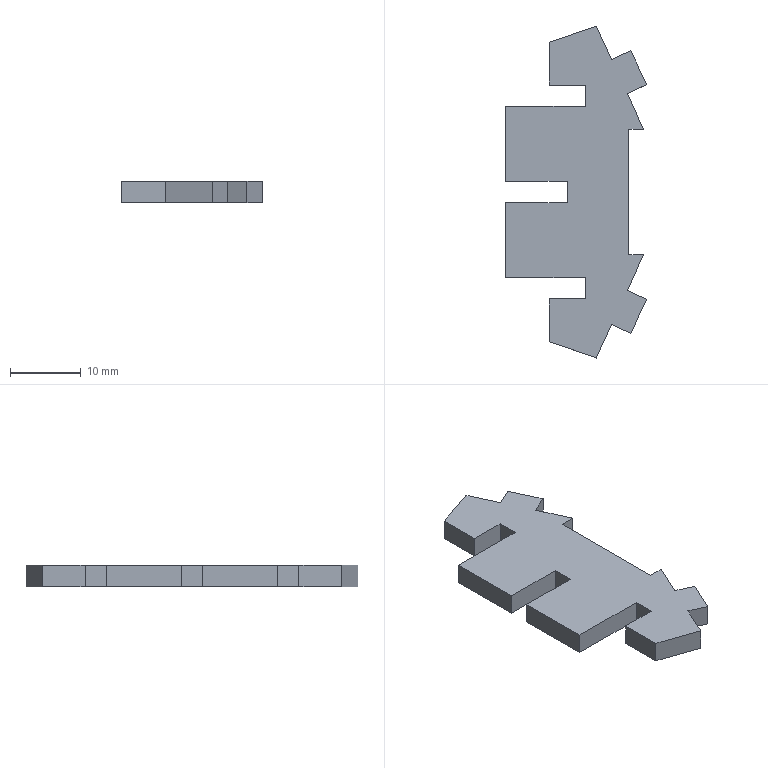Part | SolidWorks | features BaseBody 1 | 1 solid | 30 faces | box 19.907 x 46.828 x 3 mm | volume 1794 mm3 | plane 30
STEP:
#1=CARTESIAN_POINT('',(19.6,-8.833,-1.5));
#2=VERTEX_POINT('',#1);
#3=CARTESIAN_POINT('',(17.493,-8.833,-1.5));
#4=VERTEX_POINT('',#3);
#5=CARTESIAN_POINT('',(0.,-8.833,-1.5));
#6=DIRECTION('',(-1.,0.,0.));
#7=VECTOR('',#6,1000.);
#8=LINE('',#5,#7);
#9=EDGE_CURVE('',#2,#4,#8,.T.);
#10=ORIENTED_EDGE('',*,*,#9,.F.);
#11=CARTESIAN_POINT('',(17.284,-13.888,-1.5));
#12=VERTEX_POINT('',#11);
#13=CARTESIAN_POINT('',(19.544,-8.956,-1.5));
#14=DIRECTION('',(0.4166,0.9091,0.));
#15=VECTOR('',#14,1000.);
#16=LINE('',#13,#15);
#17=EDGE_CURVE('',#12,#2,#16,.T.);
#18=ORIENTED_EDGE('',*,*,#17,.F.);
#19=CARTESIAN_POINT('',(20.008,-15.138,-1.5));
#20=VERTEX_POINT('',#19);
#21=CARTESIAN_POINT('',(-2.257,-4.916,-1.5));
#22=DIRECTION('',(-0.9088,0.4172,0.));
#23=VECTOR('',#22,1000.);
#24=LINE('',#21,#23);
#25=EDGE_CURVE('',#20,#12,#24,.T.);
#26=ORIENTED_EDGE('',*,*,#25,.F.);
#27=CARTESIAN_POINT('',(17.807,-19.931,-1.5));
#28=VERTEX_POINT('',#27);
#29=CARTESIAN_POINT('',(22.265,-10.222,-1.5));
#30=DIRECTION('',(0.4172,0.9088,0.));
#31=VECTOR('',#30,1000.);
#32=LINE('',#29,#31);
#33=EDGE_CURVE('',#28,#20,#32,.T.);
#34=ORIENTED_EDGE('',*,*,#33,.F.);
#35=CARTESIAN_POINT('',(15.086,-18.681,-1.5));
#36=VERTEX_POINT('',#35);
#37=CARTESIAN_POINT('',(-4.457,-9.708,-1.5));
#38=DIRECTION('',(0.9088,-0.4172,0.));
#39=VECTOR('',#38,1000.);
#40=LINE('',#37,#39);
#41=EDGE_CURVE('',#36,#28,#40,.T.);
#42=ORIENTED_EDGE('',*,*,#41,.F.);
#43=CARTESIAN_POINT('',(12.915,-23.414,-1.5));
#44=VERTEX_POINT('',#43);
#45=CARTESIAN_POINT('',(19.544,-8.968,-1.5));
#46=DIRECTION('',(0.4171,0.9089,0.));
#47=VECTOR('',#46,1000.);
#48=LINE('',#45,#47);
#49=EDGE_CURVE('',#44,#36,#48,.T.);
#50=ORIENTED_EDGE('',*,*,#49,.F.);
#51=CARTESIAN_POINT('',(6.282,-21.117,-1.5));
#52=VERTEX_POINT('',#51);
#53=CARTESIAN_POINT('',(-5.857,-16.914,-1.5));
#54=DIRECTION('',(0.9449,-0.3272,0.));
#55=VECTOR('',#54,1000.);
#56=LINE('',#53,#55);
#57=EDGE_CURVE('',#52,#44,#56,.T.);
#58=ORIENTED_EDGE('',*,*,#57,.F.);
#59=CARTESIAN_POINT('',(6.282,-15.081,-1.5));
#60=VERTEX_POINT('',#59);
#61=CARTESIAN_POINT('',(6.282,0.,-1.5));
#62=DIRECTION('',(0.,-1.,0.));
#63=VECTOR('',#62,1000.);
#64=LINE('',#61,#63);
#65=EDGE_CURVE('',#60,#52,#64,.T.);
#66=ORIENTED_EDGE('',*,*,#65,.F.);
#67=CARTESIAN_POINT('',(11.376,-15.081,-1.5));
#68=VERTEX_POINT('',#67);
#69=CARTESIAN_POINT('',(0.,-15.081,-1.5));
#70=DIRECTION('',(-1.,0.,0.));
#71=VECTOR('',#70,1000.);
#72=LINE('',#69,#71);
#73=EDGE_CURVE('',#68,#60,#72,.T.);
#74=ORIENTED_EDGE('',*,*,#73,.F.);
#75=CARTESIAN_POINT('',(11.376,-12.086,-1.5));
#76=VERTEX_POINT('',#75);
#77=CARTESIAN_POINT('',(11.376,0.,-1.5));
#78=DIRECTION('',(0.,-1.,0.));
#79=VECTOR('',#78,1000.);
#80=LINE('',#77,#79);
#81=EDGE_CURVE('',#76,#68,#80,.T.);
#82=ORIENTED_EDGE('',*,*,#81,.F.);
#83=CARTESIAN_POINT('',(0.1003,-12.086,-1.5));
#84=VERTEX_POINT('',#83);
#85=CARTESIAN_POINT('',(0.,-12.086,-1.5));
#86=DIRECTION('',(1.,0.,0.));
#87=VECTOR('',#86,1000.);
#88=LINE('',#85,#87);
#89=EDGE_CURVE('',#84,#76,#88,.T.);
#90=ORIENTED_EDGE('',*,*,#89,.F.);
#91=CARTESIAN_POINT('',(0.1003,-1.498,-1.5));
#92=VERTEX_POINT('',#91);
#93=CARTESIAN_POINT('',(0.1003,0.,-1.5));
#94=DIRECTION('',(0.,1.,0.));
#95=VECTOR('',#94,1000.);
#96=LINE('',#93,#95);
#97=EDGE_CURVE('',#84,#92,#96,.T.);
#98=ORIENTED_EDGE('',*,*,#97,.T.);
#99=CARTESIAN_POINT('',(8.819,-1.498,-1.5));
#100=VERTEX_POINT('',#99);
#101=CARTESIAN_POINT('',(0.,-1.498,-1.5));
#102=DIRECTION('',(-1.,0.,0.));
#103=VECTOR('',#102,1000.);
#104=LINE('',#101,#103);
#105=EDGE_CURVE('',#100,#92,#104,.T.);
#106=ORIENTED_EDGE('',*,*,#105,.F.);
#107=CARTESIAN_POINT('',(8.819,1.498,-1.5));
#108=VERTEX_POINT('',#107);
#109=CARTESIAN_POINT('',(8.819,0.,-1.5));
#110=DIRECTION('',(0.,-1.,0.));
#111=VECTOR('',#110,1000.);
#112=LINE('',#109,#111);
#113=EDGE_CURVE('',#108,#100,#112,.T.);
#114=ORIENTED_EDGE('',*,*,#113,.F.);
#115=CARTESIAN_POINT('',(0.1003,1.498,-1.5));
#116=VERTEX_POINT('',#115);
#117=CARTESIAN_POINT('',(0.,1.498,-1.5));
#118=DIRECTION('',(1.,0.,0.));
#119=VECTOR('',#118,1000.);
#120=LINE('',#117,#119);
#121=EDGE_CURVE('',#116,#108,#120,.T.);
#122=ORIENTED_EDGE('',*,*,#121,.F.);
#123=CARTESIAN_POINT('',(0.1003,12.086,-1.5));
#124=VERTEX_POINT('',#123);
#125=CARTESIAN_POINT('',(0.1003,0.,-1.5));
#126=DIRECTION('',(0.,1.,0.));
#127=VECTOR('',#126,1000.);
#128=LINE('',#125,#127);
#129=EDGE_CURVE('',#116,#124,#128,.T.);
#130=ORIENTED_EDGE('',*,*,#129,.T.);
#131=CARTESIAN_POINT('',(11.376,12.086,-1.5));
#132=VERTEX_POINT('',#131);
#133=CARTESIAN_POINT('',(0.,12.086,-1.5));
#134=DIRECTION('',(-1.,0.,0.));
#135=VECTOR('',#134,1000.);
#136=LINE('',#133,#135);
#137=EDGE_CURVE('',#132,#124,#136,.T.);
#138=ORIENTED_EDGE('',*,*,#137,.F.);
#139=CARTESIAN_POINT('',(11.376,15.081,-1.5));
#140=VERTEX_POINT('',#139);
#141=CARTESIAN_POINT('',(11.376,0.,-1.5));
#142=DIRECTION('',(0.,-1.,0.));
#143=VECTOR('',#142,1000.);
#144=LINE('',#141,#143);
#145=EDGE_CURVE('',#140,#132,#144,.T.);
#146=ORIENTED_EDGE('',*,*,#145,.F.);
#147=CARTESIAN_POINT('',(6.282,15.081,-1.5));
#148=VERTEX_POINT('',#147);
#149=CARTESIAN_POINT('',(0.,15.081,-1.5));
#150=DIRECTION('',(1.,0.,0.));
#151=VECTOR('',#150,1000.);
#152=LINE('',#149,#151);
#153=EDGE_CURVE('',#148,#140,#152,.T.);
#154=ORIENTED_EDGE('',*,*,#153,.F.);
#155=CARTESIAN_POINT('',(6.282,21.117,-1.5));
#156=VERTEX_POINT('',#155);
#157=CARTESIAN_POINT('',(6.282,0.,-1.5));
#158=DIRECTION('',(0.,-1.,0.));
#159=VECTOR('',#158,1000.);
#160=LINE('',#157,#159);
#161=EDGE_CURVE('',#156,#148,#160,.T.);
#162=ORIENTED_EDGE('',*,*,#161,.F.);
#163=CARTESIAN_POINT('',(12.915,23.414,-1.5));
#164=VERTEX_POINT('',#163);
#165=CARTESIAN_POINT('',(-5.857,16.914,-1.5));
#166=DIRECTION('',(-0.9449,-0.3272,0.));
#167=VECTOR('',#166,1000.);
#168=LINE('',#165,#167);
#169=EDGE_CURVE('',#164,#156,#168,.T.);
#170=ORIENTED_EDGE('',*,*,#169,.F.);
#171=CARTESIAN_POINT('',(15.086,18.681,-1.5));
#172=VERTEX_POINT('',#171);
#173=CARTESIAN_POINT('',(19.544,8.968,-1.5));
#174=DIRECTION('',(-0.4171,0.9089,0.));
#175=VECTOR('',#174,1000.);
#176=LINE('',#173,#175);
#177=EDGE_CURVE('',#172,#164,#176,.T.);
#178=ORIENTED_EDGE('',*,*,#177,.F.);
#179=CARTESIAN_POINT('',(17.807,19.931,-1.5));
#180=VERTEX_POINT('',#179);
#181=CARTESIAN_POINT('',(-4.457,9.708,-1.5));
#182=DIRECTION('',(-0.9088,-0.4172,0.));
#183=VECTOR('',#182,1000.);
#184=LINE('',#181,#183);
#185=EDGE_CURVE('',#180,#172,#184,.T.);
#186=ORIENTED_EDGE('',*,*,#185,.F.);
#187=CARTESIAN_POINT('',(20.008,15.138,-1.5));
#188=VERTEX_POINT('',#187);
#189=CARTESIAN_POINT('',(22.265,10.222,-1.5));
#190=DIRECTION('',(-0.4172,0.9088,0.));
#191=VECTOR('',#190,1000.);
#192=LINE('',#189,#191);
#193=EDGE_CURVE('',#188,#180,#192,.T.);
#194=ORIENTED_EDGE('',*,*,#193,.F.);
#195=CARTESIAN_POINT('',(17.284,13.888,-1.5));
#196=VERTEX_POINT('',#195);
#197=CARTESIAN_POINT('',(-2.257,4.916,-1.5));
#198=DIRECTION('',(0.9088,0.4172,0.));
#199=VECTOR('',#198,1000.);
#200=LINE('',#197,#199);
#201=EDGE_CURVE('',#196,#188,#200,.T.);
#202=ORIENTED_EDGE('',*,*,#201,.F.);
#203=CARTESIAN_POINT('',(19.6,8.833,-1.5));
#204=VERTEX_POINT('',#203);
#205=CARTESIAN_POINT('',(19.544,8.956,-1.5));
#206=DIRECTION('',(-0.4166,0.9091,0.));
#207=VECTOR('',#206,1000.);
#208=LINE('',#205,#207);
#209=EDGE_CURVE('',#204,#196,#208,.T.);
#210=ORIENTED_EDGE('',*,*,#209,.F.);
#211=CARTESIAN_POINT('',(17.493,8.833,-1.5));
#212=VERTEX_POINT('',#211);
#213=CARTESIAN_POINT('',(0.,8.833,-1.5));
#214=DIRECTION('',(1.,0.,0.));
#215=VECTOR('',#214,1000.);
#216=LINE('',#213,#215);
#217=EDGE_CURVE('',#212,#204,#216,.T.);
#218=ORIENTED_EDGE('',*,*,#217,.F.);
#219=CARTESIAN_POINT('',(17.493,0.,-1.5));
#220=DIRECTION('',(0.,1.,0.));
#221=VECTOR('',#220,1000.);
#222=LINE('',#219,#221);
#223=EDGE_CURVE('',#4,#212,#222,.T.);
#224=ORIENTED_EDGE('',*,*,#223,.F.);
#225=EDGE_LOOP('',(#10,#18,#26,#34,#42,#50,#58,#66,#74,#82,#90,#98,#106,#114,#122,#130,#138,#146,#154,#162,#170,#178,#186,#194,#202,#210,#218,#224));
#226=FACE_OUTER_BOUND('',#225,.T.);
#227=CARTESIAN_POINT('',(0.,0.,-1.5));
#228=DIRECTION('',(0.,0.,1.));
#229=DIRECTION('',(1.,0.,0.));
#230=AXIS2_PLACEMENT_3D('',#227,#228,#229);
#231=PLANE('',#230);
#232=ADVANCED_FACE('',(#226),#231,.F.);
#233=CARTESIAN_POINT('',(19.6,-8.833,1.5));
#234=VERTEX_POINT('',#233);
#235=CARTESIAN_POINT('',(17.493,-8.833,1.5));
#236=VERTEX_POINT('',#235);
#237=CARTESIAN_POINT('',(0.,-8.833,1.5));
#238=DIRECTION('',(-1.,0.,0.));
#239=VECTOR('',#238,1000.);
#240=LINE('',#237,#239);
#241=EDGE_CURVE('',#234,#236,#240,.T.);
#242=ORIENTED_EDGE('',*,*,#241,.T.);
#243=CARTESIAN_POINT('',(17.493,8.833,1.5));
#244=VERTEX_POINT('',#243);
#245=CARTESIAN_POINT('',(17.493,0.,1.5));
#246=DIRECTION('',(0.,1.,0.));
#247=VECTOR('',#246,1000.);
#248=LINE('',#245,#247);
#249=EDGE_CURVE('',#236,#244,#248,.T.);
#250=ORIENTED_EDGE('',*,*,#249,.T.);
#251=CARTESIAN_POINT('',(19.6,8.833,1.5));
#252=VERTEX_POINT('',#251);
#253=CARTESIAN_POINT('',(0.,8.833,1.5));
#254=DIRECTION('',(1.,0.,0.));
#255=VECTOR('',#254,1000.);
#256=LINE('',#253,#255);
#257=EDGE_CURVE('',#244,#252,#256,.T.);
#258=ORIENTED_EDGE('',*,*,#257,.T.);
#259=CARTESIAN_POINT('',(17.284,13.888,1.5));
#260=VERTEX_POINT('',#259);
#261=CARTESIAN_POINT('',(19.544,8.956,1.5));
#262=DIRECTION('',(-0.4166,0.9091,0.));
#263=VECTOR('',#262,1000.);
#264=LINE('',#261,#263);
#265=EDGE_CURVE('',#252,#260,#264,.T.);
#266=ORIENTED_EDGE('',*,*,#265,.T.);
#267=CARTESIAN_POINT('',(20.008,15.138,1.5));
#268=VERTEX_POINT('',#267);
#269=CARTESIAN_POINT('',(-2.257,4.916,1.5));
#270=DIRECTION('',(0.9088,0.4172,0.));
#271=VECTOR('',#270,1000.);
#272=LINE('',#269,#271);
#273=EDGE_CURVE('',#260,#268,#272,.T.);
#274=ORIENTED_EDGE('',*,*,#273,.T.);
#275=CARTESIAN_POINT('',(17.807,19.931,1.5));
#276=VERTEX_POINT('',#275);
#277=CARTESIAN_POINT('',(22.265,10.222,1.5));
#278=DIRECTION('',(-0.4172,0.9088,0.));
#279=VECTOR('',#278,1000.);
#280=LINE('',#277,#279);
#281=EDGE_CURVE('',#268,#276,#280,.T.);
#282=ORIENTED_EDGE('',*,*,#281,.T.);
#283=CARTESIAN_POINT('',(15.086,18.681,1.5));
#284=VERTEX_POINT('',#283);
#285=CARTESIAN_POINT('',(-4.457,9.708,1.5));
#286=DIRECTION('',(-0.9088,-0.4172,0.));
#287=VECTOR('',#286,1000.);
#288=LINE('',#285,#287);
#289=EDGE_CURVE('',#276,#284,#288,.T.);
#290=ORIENTED_EDGE('',*,*,#289,.T.);
#291=CARTESIAN_POINT('',(12.915,23.414,1.5));
#292=VERTEX_POINT('',#291);
#293=CARTESIAN_POINT('',(19.544,8.968,1.5));
#294=DIRECTION('',(-0.4171,0.9089,0.));
#295=VECTOR('',#294,1000.);
#296=LINE('',#293,#295);
#297=EDGE_CURVE('',#284,#292,#296,.T.);
#298=ORIENTED_EDGE('',*,*,#297,.T.);
#299=CARTESIAN_POINT('',(6.282,21.117,1.5));
#300=VERTEX_POINT('',#299);
#301=CARTESIAN_POINT('',(-5.857,16.914,1.5));
#302=DIRECTION('',(-0.9449,-0.3272,0.));
#303=VECTOR('',#302,1000.);
#304=LINE('',#301,#303);
#305=EDGE_CURVE('',#292,#300,#304,.T.);
#306=ORIENTED_EDGE('',*,*,#305,.T.);
#307=CARTESIAN_POINT('',(6.282,15.081,1.5));
#308=VERTEX_POINT('',#307);
#309=CARTESIAN_POINT('',(6.282,0.,1.5));
#310=DIRECTION('',(0.,-1.,0.));
#311=VECTOR('',#310,1000.);
#312=LINE('',#309,#311);
#313=EDGE_CURVE('',#300,#308,#312,.T.);
#314=ORIENTED_EDGE('',*,*,#313,.T.);
#315=CARTESIAN_POINT('',(11.376,15.081,1.5));
#316=VERTEX_POINT('',#315);
#317=CARTESIAN_POINT('',(0.,15.081,1.5));
#318=DIRECTION('',(1.,0.,0.));
#319=VECTOR('',#318,1000.);
#320=LINE('',#317,#319);
#321=EDGE_CURVE('',#308,#316,#320,.T.);
#322=ORIENTED_EDGE('',*,*,#321,.T.);
#323=CARTESIAN_POINT('',(11.376,12.086,1.5));
#324=VERTEX_POINT('',#323);
#325=CARTESIAN_POINT('',(11.376,0.,1.5));
#326=DIRECTION('',(0.,-1.,0.));
#327=VECTOR('',#326,1000.);
#328=LINE('',#325,#327);
#329=EDGE_CURVE('',#316,#324,#328,.T.);
#330=ORIENTED_EDGE('',*,*,#329,.T.);
#331=CARTESIAN_POINT('',(0.1003,12.086,1.5));
#332=VERTEX_POINT('',#331);
#333=CARTESIAN_POINT('',(0.,12.086,1.5));
#334=DIRECTION('',(-1.,0.,0.));
#335=VECTOR('',#334,1000.);
#336=LINE('',#333,#335);
#337=EDGE_CURVE('',#324,#332,#336,.T.);
#338=ORIENTED_EDGE('',*,*,#337,.T.);
#339=CARTESIAN_POINT('',(0.1003,1.498,1.5));
#340=VERTEX_POINT('',#339);
#341=CARTESIAN_POINT('',(0.1003,0.,1.5));
#342=DIRECTION('',(0.,1.,0.));
#343=VECTOR('',#342,1000.);
#344=LINE('',#341,#343);
#345=EDGE_CURVE('',#340,#332,#344,.T.);
#346=ORIENTED_EDGE('',*,*,#345,.F.);
#347=CARTESIAN_POINT('',(8.819,1.498,1.5));
#348=VERTEX_POINT('',#347);
#349=CARTESIAN_POINT('',(0.,1.498,1.5));
#350=DIRECTION('',(1.,0.,0.));
#351=VECTOR('',#350,1000.);
#352=LINE('',#349,#351);
#353=EDGE_CURVE('',#340,#348,#352,.T.);
#354=ORIENTED_EDGE('',*,*,#353,.T.);
#355=CARTESIAN_POINT('',(8.819,-1.498,1.5));
#356=VERTEX_POINT('',#355);
#357=CARTESIAN_POINT('',(8.819,0.,1.5));
#358=DIRECTION('',(0.,-1.,0.));
#359=VECTOR('',#358,1000.);
#360=LINE('',#357,#359);
#361=EDGE_CURVE('',#348,#356,#360,.T.);
#362=ORIENTED_EDGE('',*,*,#361,.T.);
#363=CARTESIAN_POINT('',(0.1003,-1.498,1.5));
#364=VERTEX_POINT('',#363);
#365=CARTESIAN_POINT('',(0.,-1.498,1.5));
#366=DIRECTION('',(-1.,0.,0.));
#367=VECTOR('',#366,1000.);
#368=LINE('',#365,#367);
#369=EDGE_CURVE('',#356,#364,#368,.T.);
#370=ORIENTED_EDGE('',*,*,#369,.T.);
#371=CARTESIAN_POINT('',(0.1003,-12.086,1.5));
#372=VERTEX_POINT('',#371);
#373=CARTESIAN_POINT('',(0.1003,0.,1.5));
#374=DIRECTION('',(0.,1.,0.));
#375=VECTOR('',#374,1000.);
#376=LINE('',#373,#375);
#377=EDGE_CURVE('',#372,#364,#376,.T.);
#378=ORIENTED_EDGE('',*,*,#377,.F.);
#379=CARTESIAN_POINT('',(11.376,-12.086,1.5));
#380=VERTEX_POINT('',#379);
#381=CARTESIAN_POINT('',(0.,-12.086,1.5));
#382=DIRECTION('',(1.,0.,0.));
#383=VECTOR('',#382,1000.);
#384=LINE('',#381,#383);
#385=EDGE_CURVE('',#372,#380,#384,.T.);
#386=ORIENTED_EDGE('',*,*,#385,.T.);
#387=CARTESIAN_POINT('',(11.376,-15.081,1.5));
#388=VERTEX_POINT('',#387);
#389=CARTESIAN_POINT('',(11.376,0.,1.5));
#390=DIRECTION('',(0.,-1.,0.));
#391=VECTOR('',#390,1000.);
#392=LINE('',#389,#391);
#393=EDGE_CURVE('',#380,#388,#392,.T.);
#394=ORIENTED_EDGE('',*,*,#393,.T.);
#395=CARTESIAN_POINT('',(6.282,-15.081,1.5));
#396=VERTEX_POINT('',#395);
#397=CARTESIAN_POINT('',(0.,-15.081,1.5));
#398=DIRECTION('',(-1.,0.,0.));
#399=VECTOR('',#398,1000.);
#400=LINE('',#397,#399);
#401=EDGE_CURVE('',#388,#396,#400,.T.);
#402=ORIENTED_EDGE('',*,*,#401,.T.);
#403=CARTESIAN_POINT('',(6.282,-21.117,1.5));
#404=VERTEX_POINT('',#403);
#405=CARTESIAN_POINT('',(6.282,0.,1.5));
#406=DIRECTION('',(0.,-1.,0.));
#407=VECTOR('',#406,1000.);
#408=LINE('',#405,#407);
#409=EDGE_CURVE('',#396,#404,#408,.T.);
#410=ORIENTED_EDGE('',*,*,#409,.T.);
#411=CARTESIAN_POINT('',(12.915,-23.414,1.5));
#412=VERTEX_POINT('',#411);
#413=CARTESIAN_POINT('',(-5.857,-16.914,1.5));
#414=DIRECTION('',(0.9449,-0.3272,0.));
#415=VECTOR('',#414,1000.);
#416=LINE('',#413,#415);
#417=EDGE_CURVE('',#404,#412,#416,.T.);
#418=ORIENTED_EDGE('',*,*,#417,.T.);
#419=CARTESIAN_POINT('',(15.086,-18.681,1.5));
#420=VERTEX_POINT('',#419);
#421=CARTESIAN_POINT('',(19.544,-8.968,1.5));
#422=DIRECTION('',(0.4171,0.9089,0.));
#423=VECTOR('',#422,1000.);
#424=LINE('',#421,#423);
#425=EDGE_CURVE('',#412,#420,#424,.T.);
#426=ORIENTED_EDGE('',*,*,#425,.T.);
#427=CARTESIAN_POINT('',(17.807,-19.931,1.5));
#428=VERTEX_POINT('',#427);
#429=CARTESIAN_POINT('',(-4.457,-9.708,1.5));
#430=DIRECTION('',(0.9088,-0.4172,0.));
#431=VECTOR('',#430,1000.);
#432=LINE('',#429,#431);
#433=EDGE_CURVE('',#420,#428,#432,.T.);
#434=ORIENTED_EDGE('',*,*,#433,.T.);
#435=CARTESIAN_POINT('',(20.008,-15.138,1.5));
#436=VERTEX_POINT('',#435);
#437=CARTESIAN_POINT('',(22.265,-10.222,1.5));
#438=DIRECTION('',(0.4172,0.9088,0.));
#439=VECTOR('',#438,1000.);
#440=LINE('',#437,#439);
#441=EDGE_CURVE('',#428,#436,#440,.T.);
#442=ORIENTED_EDGE('',*,*,#441,.T.);
#443=CARTESIAN_POINT('',(17.284,-13.888,1.5));
#444=VERTEX_POINT('',#443);
#445=CARTESIAN_POINT('',(-2.257,-4.916,1.5));
#446=DIRECTION('',(-0.9088,0.4172,0.));
#447=VECTOR('',#446,1000.);
#448=LINE('',#445,#447);
#449=EDGE_CURVE('',#436,#444,#448,.T.);
#450=ORIENTED_EDGE('',*,*,#449,.T.);
#451=CARTESIAN_POINT('',(19.544,-8.956,1.5));
#452=DIRECTION('',(0.4166,0.9091,0.));
#453=VECTOR('',#452,1000.);
#454=LINE('',#451,#453);
#455=EDGE_CURVE('',#444,#234,#454,.T.);
#456=ORIENTED_EDGE('',*,*,#455,.T.);
#457=EDGE_LOOP('',(#242,#250,#258,#266,#274,#282,#290,#298,#306,#314,#322,#330,#338,#346,#354,#362,#370,#378,#386,#394,#402,#410,#418,#426,#434,#442,#450,#456));
#458=FACE_OUTER_BOUND('',#457,.T.);
#459=CARTESIAN_POINT('',(0.,0.,1.5));
#460=DIRECTION('',(0.,0.,1.));
#461=DIRECTION('',(1.,0.,0.));
#462=AXIS2_PLACEMENT_3D('',#459,#460,#461);
#463=PLANE('',#462);
#464=ADVANCED_FACE('',(#458),#463,.T.);
#465=ORIENTED_EDGE('',*,*,#17,.T.);
#466=CARTESIAN_POINT('',(19.6,-8.833,1.5));
#467=DIRECTION('',(0.,0.,-1.));
#468=VECTOR('',#467,1000.);
#469=LINE('',#466,#468);
#470=EDGE_CURVE('',#234,#2,#469,.T.);
#471=ORIENTED_EDGE('',*,*,#470,.F.);
#472=ORIENTED_EDGE('',*,*,#455,.F.);
#473=CARTESIAN_POINT('',(17.284,-13.888,1.5));
#474=DIRECTION('',(0.,0.,-1.));
#475=VECTOR('',#474,1000.);
#476=LINE('',#473,#475);
#477=EDGE_CURVE('',#444,#12,#476,.T.);
#478=ORIENTED_EDGE('',*,*,#477,.T.);
#479=EDGE_LOOP('',(#465,#471,#472,#478));
#480=FACE_OUTER_BOUND('',#479,.T.);
#481=CARTESIAN_POINT('',(19.544,-8.956,1.5));
#482=DIRECTION('',(-0.9091,0.4166,0.));
#483=DIRECTION('',(0.,0.,1.));
#484=AXIS2_PLACEMENT_3D('',#481,#482,#483);
#485=PLANE('',#484);
#486=ADVANCED_FACE('',(#480),#485,.F.);
#487=ORIENTED_EDGE('',*,*,#25,.T.);
#488=ORIENTED_EDGE('',*,*,#477,.F.);
#489=ORIENTED_EDGE('',*,*,#449,.F.);
#490=CARTESIAN_POINT('',(20.008,-15.138,1.5));
#491=DIRECTION('',(0.,0.,-1.));
#492=VECTOR('',#491,1000.);
#493=LINE('',#490,#492);
#494=EDGE_CURVE('',#436,#20,#493,.T.);
#495=ORIENTED_EDGE('',*,*,#494,.T.);
#496=EDGE_LOOP('',(#487,#488,#489,#495));
#497=FACE_OUTER_BOUND('',#496,.T.);
#498=CARTESIAN_POINT('',(-2.257,-4.916,1.5));
#499=DIRECTION('',(-0.4172,-0.9088,0.));
#500=DIRECTION('',(-0.9088,0.4172,0.));
#501=AXIS2_PLACEMENT_3D('',#498,#499,#500);
#502=PLANE('',#501);
#503=ADVANCED_FACE('',(#497),#502,.F.);
#504=ORIENTED_EDGE('',*,*,#33,.T.);
#505=ORIENTED_EDGE('',*,*,#494,.F.);
#506=ORIENTED_EDGE('',*,*,#441,.F.);
#507=CARTESIAN_POINT('',(17.807,-19.931,1.5));
#508=DIRECTION('',(0.,0.,-1.));
#509=VECTOR('',#508,1000.);
#510=LINE('',#507,#509);
#511=EDGE_CURVE('',#428,#28,#510,.T.);
#512=ORIENTED_EDGE('',*,*,#511,.T.);
#513=EDGE_LOOP('',(#504,#505,#506,#512));
#514=FACE_OUTER_BOUND('',#513,.T.);
#515=CARTESIAN_POINT('',(22.265,-10.222,1.5));
#516=DIRECTION('',(-0.9088,0.4172,0.));
#517=DIRECTION('',(0.,0.,1.));
#518=AXIS2_PLACEMENT_3D('',#515,#516,#517);
#519=PLANE('',#518);
#520=ADVANCED_FACE('',(#514),#519,.F.);
#521=ORIENTED_EDGE('',*,*,#41,.T.);
#522=ORIENTED_EDGE('',*,*,#511,.F.);
#523=ORIENTED_EDGE('',*,*,#433,.F.);
#524=CARTESIAN_POINT('',(15.086,-18.681,1.5));
#525=DIRECTION('',(0.,0.,-1.));
#526=VECTOR('',#525,1000.);
#527=LINE('',#524,#526);
#528=EDGE_CURVE('',#420,#36,#527,.T.);
#529=ORIENTED_EDGE('',*,*,#528,.T.);
#530=EDGE_LOOP('',(#521,#522,#523,#529));
#531=FACE_OUTER_BOUND('',#530,.T.);
#532=CARTESIAN_POINT('',(-4.457,-9.708,1.5));
#533=DIRECTION('',(0.4172,0.9088,0.));
#534=DIRECTION('',(0.,0.,-1.));
#535=AXIS2_PLACEMENT_3D('',#532,#533,#534);
#536=PLANE('',#535);
#537=ADVANCED_FACE('',(#531),#536,.F.);
#538=ORIENTED_EDGE('',*,*,#49,.T.);
#539=ORIENTED_EDGE('',*,*,#528,.F.);
#540=ORIENTED_EDGE('',*,*,#425,.F.);
#541=CARTESIAN_POINT('',(12.915,-23.414,1.5));
#542=DIRECTION('',(0.,0.,-1.));
#543=VECTOR('',#542,1000.);
#544=LINE('',#541,#543);
#545=EDGE_CURVE('',#412,#44,#544,.T.);
#546=ORIENTED_EDGE('',*,*,#545,.T.);
#547=EDGE_LOOP('',(#538,#539,#540,#546));
#548=FACE_OUTER_BOUND('',#547,.T.);
#549=CARTESIAN_POINT('',(19.544,-8.968,1.5));
#550=DIRECTION('',(-0.9089,0.4171,0.));
#551=DIRECTION('',(0.,0.,1.));
#552=AXIS2_PLACEMENT_3D('',#549,#550,#551);
#553=PLANE('',#552);
#554=ADVANCED_FACE('',(#548),#553,.F.);
#555=ORIENTED_EDGE('',*,*,#57,.T.);
#556=ORIENTED_EDGE('',*,*,#545,.F.);
#557=ORIENTED_EDGE('',*,*,#417,.F.);
#558=CARTESIAN_POINT('',(6.282,-21.117,1.5));
#559=DIRECTION('',(0.,0.,-1.));
#560=VECTOR('',#559,1000.);
#561=LINE('',#558,#560);
#562=EDGE_CURVE('',#404,#52,#561,.T.);
#563=ORIENTED_EDGE('',*,*,#562,.T.);
#564=EDGE_LOOP('',(#555,#556,#557,#563));
#565=FACE_OUTER_BOUND('',#564,.T.);
#566=CARTESIAN_POINT('',(-5.857,-16.914,1.5));
#567=DIRECTION('',(0.3272,0.9449,0.));
#568=DIRECTION('',(0.,0.,-1.));
#569=AXIS2_PLACEMENT_3D('',#566,#567,#568);
#570=PLANE('',#569);
#571=ADVANCED_FACE('',(#565),#570,.F.);
#572=ORIENTED_EDGE('',*,*,#65,.T.);
#573=ORIENTED_EDGE('',*,*,#562,.F.);
#574=ORIENTED_EDGE('',*,*,#409,.F.);
#575=CARTESIAN_POINT('',(6.282,-15.081,1.5));
#576=DIRECTION('',(0.,0.,-1.));
#577=VECTOR('',#576,1000.);
#578=LINE('',#575,#577);
#579=EDGE_CURVE('',#396,#60,#578,.T.);
#580=ORIENTED_EDGE('',*,*,#579,.T.);
#581=EDGE_LOOP('',(#572,#573,#574,#580));
#582=FACE_OUTER_BOUND('',#581,.T.);
#583=CARTESIAN_POINT('',(6.282,0.,1.5));
#584=DIRECTION('',(1.,0.,0.));
#585=DIRECTION('',(0.,1.,0.));
#586=AXIS2_PLACEMENT_3D('',#583,#584,#585);
#587=PLANE('',#586);
#588=ADVANCED_FACE('',(#582),#587,.F.);
#589=ORIENTED_EDGE('',*,*,#73,.T.);
#590=ORIENTED_EDGE('',*,*,#579,.F.);
#591=ORIENTED_EDGE('',*,*,#401,.F.);
#592=CARTESIAN_POINT('',(11.376,-15.081,1.5));
#593=DIRECTION('',(0.,0.,-1.));
#594=VECTOR('',#593,1000.);
#595=LINE('',#592,#594);
#596=EDGE_CURVE('',#388,#68,#595,.T.);
#597=ORIENTED_EDGE('',*,*,#596,.T.);
#598=EDGE_LOOP('',(#589,#590,#591,#597));
#599=FACE_OUTER_BOUND('',#598,.T.);
#600=CARTESIAN_POINT('',(0.,-15.081,1.5));
#601=DIRECTION('',(0.,-1.,0.));
#602=DIRECTION('',(0.,0.,-1.));
#603=AXIS2_PLACEMENT_3D('',#600,#601,#602);
#604=PLANE('',#603);
#605=ADVANCED_FACE('',(#599),#604,.F.);
#606=ORIENTED_EDGE('',*,*,#81,.T.);
#607=ORIENTED_EDGE('',*,*,#596,.F.);
#608=ORIENTED_EDGE('',*,*,#393,.F.);
#609=CARTESIAN_POINT('',(11.376,-12.086,1.5));
#610=DIRECTION('',(0.,0.,-1.));
#611=VECTOR('',#610,1000.);
#612=LINE('',#609,#611);
#613=EDGE_CURVE('',#380,#76,#612,.T.);
#614=ORIENTED_EDGE('',*,*,#613,.T.);
#615=EDGE_LOOP('',(#606,#607,#608,#614));
#616=FACE_OUTER_BOUND('',#615,.T.);
#617=CARTESIAN_POINT('',(11.376,0.,1.5));
#618=DIRECTION('',(1.,0.,0.));
#619=DIRECTION('',(0.,1.,0.));
#620=AXIS2_PLACEMENT_3D('',#617,#618,#619);
#621=PLANE('',#620);
#622=ADVANCED_FACE('',(#616),#621,.F.);
#623=ORIENTED_EDGE('',*,*,#89,.T.);
#624=ORIENTED_EDGE('',*,*,#613,.F.);
#625=ORIENTED_EDGE('',*,*,#385,.F.);
#626=CARTESIAN_POINT('',(0.1003,-12.086,1.5));
#627=DIRECTION('',(0.,0.,-1.));
#628=VECTOR('',#627,1000.);
#629=LINE('',#626,#628);
#630=EDGE_CURVE('',#372,#84,#629,.T.);
#631=ORIENTED_EDGE('',*,*,#630,.T.);
#632=EDGE_LOOP('',(#623,#624,#625,#631));
#633=FACE_OUTER_BOUND('',#632,.T.);
#634=CARTESIAN_POINT('',(0.,-12.086,1.5));
#635=DIRECTION('',(0.,1.,0.));
#636=DIRECTION('',(1.,0.,0.));
#637=AXIS2_PLACEMENT_3D('',#634,#635,#636);
#638=PLANE('',#637);
#639=ADVANCED_FACE('',(#633),#638,.F.);
#640=ORIENTED_EDGE('',*,*,#97,.F.);
#641=ORIENTED_EDGE('',*,*,#630,.F.);
#642=ORIENTED_EDGE('',*,*,#377,.T.);
#643=CARTESIAN_POINT('',(0.1003,-1.498,1.5));
#644=DIRECTION('',(0.,0.,-1.));
#645=VECTOR('',#644,1000.);
#646=LINE('',#643,#645);
#647=EDGE_CURVE('',#364,#92,#646,.T.);
#648=ORIENTED_EDGE('',*,*,#647,.T.);
#649=EDGE_LOOP('',(#640,#641,#642,#648));
#650=FACE_OUTER_BOUND('',#649,.T.);
#651=CARTESIAN_POINT('',(0.1003,0.,1.5));
#652=DIRECTION('',(-1.,0.,0.));
#653=DIRECTION('',(0.,0.,1.));
#654=AXIS2_PLACEMENT_3D('',#651,#652,#653);
#655=PLANE('',#654);
#656=ADVANCED_FACE('',(#650),#655,.T.);
#657=ORIENTED_EDGE('',*,*,#105,.T.);
#658=ORIENTED_EDGE('',*,*,#647,.F.);
#659=ORIENTED_EDGE('',*,*,#369,.F.);
#660=CARTESIAN_POINT('',(8.819,-1.498,1.5));
#661=DIRECTION('',(0.,0.,-1.));
#662=VECTOR('',#661,1000.);
#663=LINE('',#660,#662);
#664=EDGE_CURVE('',#356,#100,#663,.T.);
#665=ORIENTED_EDGE('',*,*,#664,.T.);
#666=EDGE_LOOP('',(#657,#658,#659,#665));
#667=FACE_OUTER_BOUND('',#666,.T.);
#668=CARTESIAN_POINT('',(0.,-1.498,1.5));
#669=DIRECTION('',(0.,-1.,0.));
#670=DIRECTION('',(0.,0.,-1.));
#671=AXIS2_PLACEMENT_3D('',#668,#669,#670);
#672=PLANE('',#671);
#673=ADVANCED_FACE('',(#667),#672,.F.);
#674=ORIENTED_EDGE('',*,*,#113,.T.);
#675=ORIENTED_EDGE('',*,*,#664,.F.);
#676=ORIENTED_EDGE('',*,*,#361,.F.);
#677=CARTESIAN_POINT('',(8.819,1.498,1.5));
#678=DIRECTION('',(0.,0.,-1.));
#679=VECTOR('',#678,1000.);
#680=LINE('',#677,#679);
#681=EDGE_CURVE('',#348,#108,#680,.T.);
#682=ORIENTED_EDGE('',*,*,#681,.T.);
#683=EDGE_LOOP('',(#674,#675,#676,#682));
#684=FACE_OUTER_BOUND('',#683,.T.);
#685=CARTESIAN_POINT('',(8.819,0.,1.5));
#686=DIRECTION('',(1.,0.,0.));
#687=DIRECTION('',(0.,1.,0.));
#688=AXIS2_PLACEMENT_3D('',#685,#686,#687);
#689=PLANE('',#688);
#690=ADVANCED_FACE('',(#684),#689,.F.);
#691=ORIENTED_EDGE('',*,*,#121,.T.);
#692=ORIENTED_EDGE('',*,*,#681,.F.);
#693=ORIENTED_EDGE('',*,*,#353,.F.);
#694=CARTESIAN_POINT('',(0.1003,1.498,1.5));
#695=DIRECTION('',(0.,0.,-1.));
#696=VECTOR('',#695,1000.);
#697=LINE('',#694,#696);
#698=EDGE_CURVE('',#340,#116,#697,.T.);
#699=ORIENTED_EDGE('',*,*,#698,.T.);
#700=EDGE_LOOP('',(#691,#692,#693,#699));
#701=FACE_OUTER_BOUND('',#700,.T.);
#702=CARTESIAN_POINT('',(0.,1.498,1.5));
#703=DIRECTION('',(0.,1.,0.));
#704=DIRECTION('',(1.,0.,0.));
#705=AXIS2_PLACEMENT_3D('',#702,#703,#704);
#706=PLANE('',#705);
#707=ADVANCED_FACE('',(#701),#706,.F.);
#708=ORIENTED_EDGE('',*,*,#129,.F.);
#709=ORIENTED_EDGE('',*,*,#698,.F.);
#710=ORIENTED_EDGE('',*,*,#345,.T.);
#711=CARTESIAN_POINT('',(0.1003,12.086,1.5));
#712=DIRECTION('',(0.,0.,-1.));
#713=VECTOR('',#712,1000.);
#714=LINE('',#711,#713);
#715=EDGE_CURVE('',#332,#124,#714,.T.);
#716=ORIENTED_EDGE('',*,*,#715,.T.);
#717=EDGE_LOOP('',(#708,#709,#710,#716));
#718=FACE_OUTER_BOUND('',#717,.T.);
#719=CARTESIAN_POINT('',(0.1003,0.,1.5));
#720=DIRECTION('',(-1.,0.,0.));
#721=DIRECTION('',(0.,0.,1.));
#722=AXIS2_PLACEMENT_3D('',#719,#720,#721);
#723=PLANE('',#722);
#724=ADVANCED_FACE('',(#718),#723,.T.);
#725=ORIENTED_EDGE('',*,*,#137,.T.);
#726=ORIENTED_EDGE('',*,*,#715,.F.);
#727=ORIENTED_EDGE('',*,*,#337,.F.);
#728=CARTESIAN_POINT('',(11.376,12.086,1.5));
#729=DIRECTION('',(0.,0.,-1.));
#730=VECTOR('',#729,1000.);
#731=LINE('',#728,#730);
#732=EDGE_CURVE('',#324,#132,#731,.T.);
#733=ORIENTED_EDGE('',*,*,#732,.T.);
#734=EDGE_LOOP('',(#725,#726,#727,#733));
#735=FACE_OUTER_BOUND('',#734,.T.);
#736=CARTESIAN_POINT('',(0.,12.086,1.5));
#737=DIRECTION('',(0.,-1.,0.));
#738=DIRECTION('',(0.,0.,-1.));
#739=AXIS2_PLACEMENT_3D('',#736,#737,#738);
#740=PLANE('',#739);
#741=ADVANCED_FACE('',(#735),#740,.F.);
#742=ORIENTED_EDGE('',*,*,#145,.T.);
#743=ORIENTED_EDGE('',*,*,#732,.F.);
#744=ORIENTED_EDGE('',*,*,#329,.F.);
#745=CARTESIAN_POINT('',(11.376,15.081,1.5));
#746=DIRECTION('',(0.,0.,-1.));
#747=VECTOR('',#746,1000.);
#748=LINE('',#745,#747);
#749=EDGE_CURVE('',#316,#140,#748,.T.);
#750=ORIENTED_EDGE('',*,*,#749,.T.);
#751=EDGE_LOOP('',(#742,#743,#744,#750));
#752=FACE_OUTER_BOUND('',#751,.T.);
#753=CARTESIAN_POINT('',(11.376,0.,1.5));
#754=DIRECTION('',(1.,0.,0.));
#755=DIRECTION('',(0.,1.,0.));
#756=AXIS2_PLACEMENT_3D('',#753,#754,#755);
#757=PLANE('',#756);
#758=ADVANCED_FACE('',(#752),#757,.F.);
#759=ORIENTED_EDGE('',*,*,#153,.T.);
#760=ORIENTED_EDGE('',*,*,#749,.F.);
#761=ORIENTED_EDGE('',*,*,#321,.F.);
#762=CARTESIAN_POINT('',(6.282,15.081,1.5));
#763=DIRECTION('',(0.,0.,-1.));
#764=VECTOR('',#763,1000.);
#765=LINE('',#762,#764);
#766=EDGE_CURVE('',#308,#148,#765,.T.);
#767=ORIENTED_EDGE('',*,*,#766,.T.);
#768=EDGE_LOOP('',(#759,#760,#761,#767));
#769=FACE_OUTER_BOUND('',#768,.T.);
#770=CARTESIAN_POINT('',(0.,15.081,1.5));
#771=DIRECTION('',(0.,1.,0.));
#772=DIRECTION('',(1.,0.,0.));
#773=AXIS2_PLACEMENT_3D('',#770,#771,#772);
#774=PLANE('',#773);
#775=ADVANCED_FACE('',(#769),#774,.F.);
#776=ORIENTED_EDGE('',*,*,#161,.T.);
#777=ORIENTED_EDGE('',*,*,#766,.F.);
#778=ORIENTED_EDGE('',*,*,#313,.F.);
#779=CARTESIAN_POINT('',(6.282,21.117,1.5));
#780=DIRECTION('',(0.,0.,-1.));
#781=VECTOR('',#780,1000.);
#782=LINE('',#779,#781);
#783=EDGE_CURVE('',#300,#156,#782,.T.);
#784=ORIENTED_EDGE('',*,*,#783,.T.);
#785=EDGE_LOOP('',(#776,#777,#778,#784));
#786=FACE_OUTER_BOUND('',#785,.T.);
#787=CARTESIAN_POINT('',(6.282,0.,1.5));
#788=DIRECTION('',(1.,0.,0.));
#789=DIRECTION('',(0.,1.,0.));
#790=AXIS2_PLACEMENT_3D('',#787,#788,#789);
#791=PLANE('',#790);
#792=ADVANCED_FACE('',(#786),#791,.F.);
#793=ORIENTED_EDGE('',*,*,#169,.T.);
#794=ORIENTED_EDGE('',*,*,#783,.F.);
#795=ORIENTED_EDGE('',*,*,#305,.F.);
#796=CARTESIAN_POINT('',(12.915,23.414,1.5));
#797=DIRECTION('',(0.,0.,-1.));
#798=VECTOR('',#797,1000.);
#799=LINE('',#796,#798);
#800=EDGE_CURVE('',#292,#164,#799,.T.);
#801=ORIENTED_EDGE('',*,*,#800,.T.);
#802=EDGE_LOOP('',(#793,#794,#795,#801));
#803=FACE_OUTER_BOUND('',#802,.T.);
#804=CARTESIAN_POINT('',(-5.857,16.914,1.5));
#805=DIRECTION('',(0.3272,-0.9449,0.));
#806=DIRECTION('',(0.,0.,-1.));
#807=AXIS2_PLACEMENT_3D('',#804,#805,#806);
#808=PLANE('',#807);
#809=ADVANCED_FACE('',(#803),#808,.F.);
#810=ORIENTED_EDGE('',*,*,#177,.T.);
#811=ORIENTED_EDGE('',*,*,#800,.F.);
#812=ORIENTED_EDGE('',*,*,#297,.F.);
#813=CARTESIAN_POINT('',(15.086,18.681,1.5));
#814=DIRECTION('',(0.,0.,-1.));
#815=VECTOR('',#814,1000.);
#816=LINE('',#813,#815);
#817=EDGE_CURVE('',#284,#172,#816,.T.);
#818=ORIENTED_EDGE('',*,*,#817,.T.);
#819=EDGE_LOOP('',(#810,#811,#812,#818));
#820=FACE_OUTER_BOUND('',#819,.T.);
#821=CARTESIAN_POINT('',(19.544,8.968,1.5));
#822=DIRECTION('',(-0.9089,-0.4171,0.));
#823=DIRECTION('',(-0.4171,0.9089,0.));
#824=AXIS2_PLACEMENT_3D('',#821,#822,#823);
#825=PLANE('',#824);
#826=ADVANCED_FACE('',(#820),#825,.F.);
#827=ORIENTED_EDGE('',*,*,#185,.T.);
#828=ORIENTED_EDGE('',*,*,#817,.F.);
#829=ORIENTED_EDGE('',*,*,#289,.F.);
#830=CARTESIAN_POINT('',(17.807,19.931,1.5));
#831=DIRECTION('',(0.,0.,-1.));
#832=VECTOR('',#831,1000.);
#833=LINE('',#830,#832);
#834=EDGE_CURVE('',#276,#180,#833,.T.);
#835=ORIENTED_EDGE('',*,*,#834,.T.);
#836=EDGE_LOOP('',(#827,#828,#829,#835));
#837=FACE_OUTER_BOUND('',#836,.T.);
#838=CARTESIAN_POINT('',(-4.457,9.708,1.5));
#839=DIRECTION('',(0.4172,-0.9088,0.));
#840=DIRECTION('',(0.,0.,-1.));
#841=AXIS2_PLACEMENT_3D('',#838,#839,#840);
#842=PLANE('',#841);
#843=ADVANCED_FACE('',(#837),#842,.F.);
#844=ORIENTED_EDGE('',*,*,#193,.T.);
#845=ORIENTED_EDGE('',*,*,#834,.F.);
#846=ORIENTED_EDGE('',*,*,#281,.F.);
#847=CARTESIAN_POINT('',(20.008,15.138,1.5));
#848=DIRECTION('',(0.,0.,-1.));
#849=VECTOR('',#848,1000.);
#850=LINE('',#847,#849);
#851=EDGE_CURVE('',#268,#188,#850,.T.);
#852=ORIENTED_EDGE('',*,*,#851,.T.);
#853=EDGE_LOOP('',(#844,#845,#846,#852));
#854=FACE_OUTER_BOUND('',#853,.T.);
#855=CARTESIAN_POINT('',(22.265,10.222,1.5));
#856=DIRECTION('',(-0.9088,-0.4172,0.));
#857=DIRECTION('',(-0.4172,0.9088,0.));
#858=AXIS2_PLACEMENT_3D('',#855,#856,#857);
#859=PLANE('',#858);
#860=ADVANCED_FACE('',(#854),#859,.F.);
#861=ORIENTED_EDGE('',*,*,#201,.T.);
#862=ORIENTED_EDGE('',*,*,#851,.F.);
#863=ORIENTED_EDGE('',*,*,#273,.F.);
#864=CARTESIAN_POINT('',(17.284,13.888,1.5));
#865=DIRECTION('',(0.,0.,-1.));
#866=VECTOR('',#865,1000.);
#867=LINE('',#864,#866);
#868=EDGE_CURVE('',#260,#196,#867,.T.);
#869=ORIENTED_EDGE('',*,*,#868,.T.);
#870=EDGE_LOOP('',(#861,#862,#863,#869));
#871=FACE_OUTER_BOUND('',#870,.T.);
#872=CARTESIAN_POINT('',(-2.257,4.916,1.5));
#873=DIRECTION('',(-0.4172,0.9088,0.));
#874=DIRECTION('',(0.,0.,1.));
#875=AXIS2_PLACEMENT_3D('',#872,#873,#874);
#876=PLANE('',#875);
#877=ADVANCED_FACE('',(#871),#876,.F.);
#878=ORIENTED_EDGE('',*,*,#209,.T.);
#879=ORIENTED_EDGE('',*,*,#868,.F.);
#880=ORIENTED_EDGE('',*,*,#265,.F.);
#881=CARTESIAN_POINT('',(19.6,8.833,1.5));
#882=DIRECTION('',(0.,0.,-1.));
#883=VECTOR('',#882,1000.);
#884=LINE('',#881,#883);
#885=EDGE_CURVE('',#252,#204,#884,.T.);
#886=ORIENTED_EDGE('',*,*,#885,.T.);
#887=EDGE_LOOP('',(#878,#879,#880,#886));
#888=FACE_OUTER_BOUND('',#887,.T.);
#889=CARTESIAN_POINT('',(19.544,8.956,1.5));
#890=DIRECTION('',(-0.9091,-0.4166,0.));
#891=DIRECTION('',(-0.4166,0.9091,0.));
#892=AXIS2_PLACEMENT_3D('',#889,#890,#891);
#893=PLANE('',#892);
#894=ADVANCED_FACE('',(#888),#893,.F.);
#895=ORIENTED_EDGE('',*,*,#217,.T.);
#896=ORIENTED_EDGE('',*,*,#885,.F.);
#897=ORIENTED_EDGE('',*,*,#257,.F.);
#898=CARTESIAN_POINT('',(17.493,8.833,1.5));
#899=DIRECTION('',(0.,0.,-1.));
#900=VECTOR('',#899,1000.);
#901=LINE('',#898,#900);
#902=EDGE_CURVE('',#244,#212,#901,.T.);
#903=ORIENTED_EDGE('',*,*,#902,.T.);
#904=EDGE_LOOP('',(#895,#896,#897,#903));
#905=FACE_OUTER_BOUND('',#904,.T.);
#906=CARTESIAN_POINT('',(0.,8.833,1.5));
#907=DIRECTION('',(0.,1.,0.));
#908=DIRECTION('',(1.,0.,0.));
#909=AXIS2_PLACEMENT_3D('',#906,#907,#908);
#910=PLANE('',#909);
#911=ADVANCED_FACE('',(#905),#910,.F.);
#912=ORIENTED_EDGE('',*,*,#223,.T.);
#913=ORIENTED_EDGE('',*,*,#902,.F.);
#914=ORIENTED_EDGE('',*,*,#249,.F.);
#915=CARTESIAN_POINT('',(17.493,-8.833,1.5));
#916=DIRECTION('',(0.,0.,-1.));
#917=VECTOR('',#916,1000.);
#918=LINE('',#915,#917);
#919=EDGE_CURVE('',#236,#4,#918,.T.);
#920=ORIENTED_EDGE('',*,*,#919,.T.);
#921=EDGE_LOOP('',(#912,#913,#914,#920));
#922=FACE_OUTER_BOUND('',#921,.T.);
#923=CARTESIAN_POINT('',(17.493,0.,1.5));
#924=DIRECTION('',(-1.,0.,0.));
#925=DIRECTION('',(0.,0.,1.));
#926=AXIS2_PLACEMENT_3D('',#923,#924,#925);
#927=PLANE('',#926);
#928=ADVANCED_FACE('',(#922),#927,.F.);
#929=ORIENTED_EDGE('',*,*,#9,.T.);
#930=ORIENTED_EDGE('',*,*,#919,.F.);
#931=ORIENTED_EDGE('',*,*,#241,.F.);
#932=ORIENTED_EDGE('',*,*,#470,.T.);
#933=EDGE_LOOP('',(#929,#930,#931,#932));
#934=FACE_OUTER_BOUND('',#933,.T.);
#935=CARTESIAN_POINT('',(0.,-8.833,1.5));
#936=DIRECTION('',(0.,-1.,0.));
#937=DIRECTION('',(0.,0.,-1.));
#938=AXIS2_PLACEMENT_3D('',#935,#936,#937);
#939=PLANE('',#938);
#940=ADVANCED_FACE('',(#934),#939,.F.);
#941=CLOSED_SHELL('',(#232,#464,#486,#503,#520,#537,#554,#571,#588,#605,#622,#639,#656,#673,#690,#707,#724,#741,#758,#775,#792,#809,#826,#843,#860,#877,#894,#911,#928,#940));
#942=MANIFOLD_SOLID_BREP('',#941);
#943=CARTESIAN_POINT('',(0.,0.,0.));
#944=DIRECTION('',(0.,0.,1.));
#945=DIRECTION('',(1.,0.,0.));
#946=AXIS2_PLACEMENT_3D('',#943,#944,#945);
#947=(LENGTH_UNIT()NAMED_UNIT(*)SI_UNIT(.MILLI.,.METRE.));
#948=UNCERTAINTY_MEASURE_WITH_UNIT(LENGTH_MEASURE(0.00001),#947,'','');
#949=(NAMED_UNIT(*)PLANE_ANGLE_UNIT()SI_UNIT($,.RADIAN.));
#950=(NAMED_UNIT(*)SI_UNIT($,.STERADIAN.)SOLID_ANGLE_UNIT());
#951=(GEOMETRIC_REPRESENTATION_CONTEXT(3)GLOBAL_UNCERTAINTY_ASSIGNED_CONTEXT((#948))GLOBAL_UNIT_ASSIGNED_CONTEXT((#947,#949,#950))REPRESENTATION_CONTEXT('',''));
#952=ADVANCED_BREP_SHAPE_REPRESENTATION('',(#942,#946),#951);